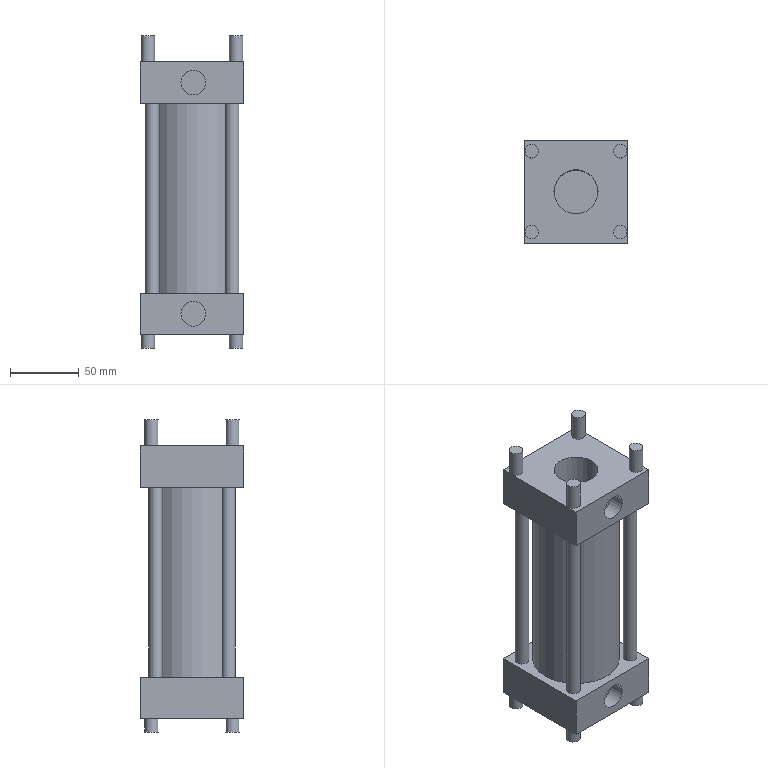Part | NX | features solid 2 | 1 solid | 39 faces | box 75 x 75 x 227 mm | volume 665796 mm3 | plane 23 | cylinder 16 | commonest cylinder face diameters 9.874 x12 18 x2 32 x1 63 x1
STEP:
#1=CARTESIAN_POINT('',(-34.06,-86.406,-135.));
#2=VERTEX_POINT('',#1);
#3=CARTESIAN_POINT('',(-29.124,-86.406,-135.));
#4=DIRECTION('',(0.,0.,-1.));
#5=DIRECTION('',(-1.,0.,0.));
#6=AXIS2_PLACEMENT_3D('',#3,#4,#5);
#7=CIRCLE('',#6,4.937);
#8=EDGE_CURVE('',#2,#2,#7,.T.);
#9=ORIENTED_EDGE('',*,*,#8,.F.);
#10=EDGE_LOOP('',(#9));
#11=FACE_BOUND('',#10,.T.);
#12=CARTESIAN_POINT('',(-24.187,-33.594,-135.));
#13=VERTEX_POINT('',#12);
#14=CARTESIAN_POINT('',(-29.124,-33.594,-135.));
#15=DIRECTION('',(0.,0.,1.));
#16=DIRECTION('',(1.,0.,0.));
#17=AXIS2_PLACEMENT_3D('',#14,#15,#16);
#18=CIRCLE('',#17,4.937);
#19=EDGE_CURVE('',#13,#13,#18,.T.);
#20=ORIENTED_EDGE('',*,*,#19,.T.);
#21=EDGE_LOOP('',(#20));
#22=FACE_BOUND('',#21,.T.);
#23=CARTESIAN_POINT('',(37.5,-97.5,-135.));
#24=VERTEX_POINT('',#23);
#25=CARTESIAN_POINT('',(-37.5,-97.5,-135.));
#26=VERTEX_POINT('',#25);
#27=CARTESIAN_POINT('',(-41.,-97.5,-135.));
#28=DIRECTION('',(-1.,0.,0.));
#29=VECTOR('',#28,1000.);
#30=LINE('',#27,#29);
#31=EDGE_CURVE('',#24,#26,#30,.T.);
#32=ORIENTED_EDGE('',*,*,#31,.T.);
#33=CARTESIAN_POINT('',(-37.5,-22.5,-135.));
#34=VERTEX_POINT('',#33);
#35=CARTESIAN_POINT('',(-37.5,-60.,-135.));
#36=DIRECTION('',(0.,1.,0.));
#37=VECTOR('',#36,1000.);
#38=LINE('',#35,#37);
#39=EDGE_CURVE('',#26,#34,#38,.T.);
#40=ORIENTED_EDGE('',*,*,#39,.T.);
#41=CARTESIAN_POINT('',(37.5,-22.5,-135.));
#42=VERTEX_POINT('',#41);
#43=CARTESIAN_POINT('',(-41.,-22.5,-135.));
#44=DIRECTION('',(-1.,0.,0.));
#45=VECTOR('',#44,1000.);
#46=LINE('',#43,#45);
#47=EDGE_CURVE('',#42,#34,#46,.T.);
#48=ORIENTED_EDGE('',*,*,#47,.F.);
#49=CARTESIAN_POINT('',(37.5,-60.,-135.));
#50=DIRECTION('',(0.,-1.,0.));
#51=VECTOR('',#50,1000.);
#52=LINE('',#49,#51);
#53=EDGE_CURVE('',#42,#24,#52,.T.);
#54=ORIENTED_EDGE('',*,*,#53,.T.);
#55=EDGE_LOOP('',(#32,#40,#48,#54));
#56=FACE_BOUND('',#55,.T.);
#57=CARTESIAN_POINT('',(34.06,-33.594,-135.));
#58=VERTEX_POINT('',#57);
#59=CARTESIAN_POINT('',(29.124,-33.594,-135.));
#60=DIRECTION('',(0.,0.,-1.));
#61=DIRECTION('',(1.,0.,0.));
#62=AXIS2_PLACEMENT_3D('',#59,#60,#61);
#63=CIRCLE('',#62,4.937);
#64=EDGE_CURVE('',#58,#58,#63,.T.);
#65=ORIENTED_EDGE('',*,*,#64,.F.);
#66=EDGE_LOOP('',(#65));
#67=FACE_BOUND('',#66,.T.);
#68=CARTESIAN_POINT('',(34.06,-86.406,-135.));
#69=VERTEX_POINT('',#68);
#70=CARTESIAN_POINT('',(29.124,-86.406,-135.));
#71=DIRECTION('',(0.,0.,1.));
#72=DIRECTION('',(1.,0.,0.));
#73=AXIS2_PLACEMENT_3D('',#70,#71,#72);
#74=CIRCLE('',#73,4.937);
#75=EDGE_CURVE('',#69,#69,#74,.T.);
#76=ORIENTED_EDGE('',*,*,#75,.T.);
#77=EDGE_LOOP('',(#76));
#78=FACE_BOUND('',#77,.T.);
#79=CARTESIAN_POINT('',(31.5,-60.,-135.));
#80=VERTEX_POINT('',#79);
#81=CARTESIAN_POINT('',(0.,-60.,-135.));
#82=DIRECTION('',(0.,0.,1.));
#83=DIRECTION('',(1.,0.,0.));
#84=AXIS2_PLACEMENT_3D('',#81,#82,#83);
#85=CIRCLE('',#84,31.5);
#86=EDGE_CURVE('',#80,#80,#85,.F.);
#87=ORIENTED_EDGE('',*,*,#86,.F.);
#88=EDGE_LOOP('',(#87));
#89=FACE_BOUND('',#88,.T.);
#90=CARTESIAN_POINT('',(-41.,-101.,-135.));
#91=DIRECTION('',(0.,0.,1.));
#92=DIRECTION('',(1.,0.,0.));
#93=AXIS2_PLACEMENT_3D('',#90,#91,#92);
#94=PLANE('',#93);
#95=ADVANCED_FACE('',(#11,#22,#56,#67,#78,#89),#94,.F.);
#96=CARTESIAN_POINT('',(-8.,-97.5,-120.));
#97=VERTEX_POINT('',#96);
#98=CARTESIAN_POINT('',(1.,-97.5,-120.));
#99=DIRECTION('',(0.,1.,0.));
#100=DIRECTION('',(-1.,0.,0.));
#101=AXIS2_PLACEMENT_3D('',#98,#99,#100);
#102=CIRCLE('',#101,9.);
#103=EDGE_CURVE('',#97,#97,#102,.T.);
#104=ORIENTED_EDGE('',*,*,#103,.T.);
#105=EDGE_LOOP('',(#104));
#106=FACE_BOUND('',#105,.T.);
#107=CARTESIAN_POINT('',(37.5,-97.5,-105.));
#108=VERTEX_POINT('',#107);
#109=CARTESIAN_POINT('',(-37.5,-97.5,-105.));
#110=VERTEX_POINT('',#109);
#111=CARTESIAN_POINT('',(-41.,-97.5,-105.));
#112=DIRECTION('',(-1.,0.,0.));
#113=VECTOR('',#112,1000.);
#114=LINE('',#111,#113);
#115=EDGE_CURVE('',#108,#110,#114,.T.);
#116=ORIENTED_EDGE('',*,*,#115,.T.);
#117=CARTESIAN_POINT('',(-37.5,-97.5,-135.));
#118=DIRECTION('',(0.,0.,1.));
#119=VECTOR('',#118,1000.);
#120=LINE('',#117,#119);
#121=EDGE_CURVE('',#26,#110,#120,.T.);
#122=ORIENTED_EDGE('',*,*,#121,.F.);
#123=ORIENTED_EDGE('',*,*,#31,.F.);
#124=CARTESIAN_POINT('',(37.5,-97.5,-135.));
#125=DIRECTION('',(0.,0.,1.));
#126=VECTOR('',#125,1000.);
#127=LINE('',#124,#126);
#128=EDGE_CURVE('',#24,#108,#127,.T.);
#129=ORIENTED_EDGE('',*,*,#128,.T.);
#130=EDGE_LOOP('',(#116,#122,#123,#129));
#131=FACE_BOUND('',#130,.T.);
#132=CARTESIAN_POINT('',(41.,-97.5,-135.));
#133=DIRECTION('',(0.,1.,0.));
#134=DIRECTION('',(-1.,0.,0.));
#135=AXIS2_PLACEMENT_3D('',#132,#133,#134);
#136=PLANE('',#135);
#137=ADVANCED_FACE('',(#106,#131),#136,.F.);
#138=CARTESIAN_POINT('',(37.5,-22.5,-105.));
#139=VERTEX_POINT('',#138);
#140=CARTESIAN_POINT('',(37.5,-101.,-105.));
#141=DIRECTION('',(0.,1.,0.));
#142=VECTOR('',#141,1000.);
#143=LINE('',#140,#142);
#144=EDGE_CURVE('',#108,#139,#143,.T.);
#145=ORIENTED_EDGE('',*,*,#144,.F.);
#146=ORIENTED_EDGE('',*,*,#128,.F.);
#147=ORIENTED_EDGE('',*,*,#53,.F.);
#148=CARTESIAN_POINT('',(37.5,-22.5,-135.));
#149=DIRECTION('',(0.,0.,1.));
#150=VECTOR('',#149,1000.);
#151=LINE('',#148,#150);
#152=EDGE_CURVE('',#42,#139,#151,.T.);
#153=ORIENTED_EDGE('',*,*,#152,.T.);
#154=EDGE_LOOP('',(#145,#146,#147,#153));
#155=FACE_BOUND('',#154,.T.);
#156=CARTESIAN_POINT('',(37.5,-60.,-135.));
#157=DIRECTION('',(1.,0.,0.));
#158=DIRECTION('',(0.,1.,0.));
#159=AXIS2_PLACEMENT_3D('',#156,#157,#158);
#160=PLANE('',#159);
#161=ADVANCED_FACE('',(#155),#160,.T.);
#162=CARTESIAN_POINT('',(-37.5,-22.5,-105.));
#163=VERTEX_POINT('',#162);
#164=CARTESIAN_POINT('',(-41.,-22.5,-105.));
#165=DIRECTION('',(1.,0.,0.));
#166=VECTOR('',#165,1000.);
#167=LINE('',#164,#166);
#168=EDGE_CURVE('',#163,#139,#167,.T.);
#169=ORIENTED_EDGE('',*,*,#168,.T.);
#170=ORIENTED_EDGE('',*,*,#152,.F.);
#171=ORIENTED_EDGE('',*,*,#47,.T.);
#172=CARTESIAN_POINT('',(-37.5,-22.5,-135.));
#173=DIRECTION('',(0.,0.,1.));
#174=VECTOR('',#173,1000.);
#175=LINE('',#172,#174);
#176=EDGE_CURVE('',#34,#163,#175,.T.);
#177=ORIENTED_EDGE('',*,*,#176,.T.);
#178=EDGE_LOOP('',(#169,#170,#171,#177));
#179=FACE_BOUND('',#178,.T.);
#180=CARTESIAN_POINT('',(-41.,-22.5,-135.));
#181=DIRECTION('',(0.,-1.,0.));
#182=DIRECTION('',(0.,0.,-1.));
#183=AXIS2_PLACEMENT_3D('',#180,#181,#182);
#184=PLANE('',#183);
#185=ADVANCED_FACE('',(#179),#184,.F.);
#186=CARTESIAN_POINT('',(-37.5,-101.,-105.));
#187=DIRECTION('',(0.,-1.,0.));
#188=VECTOR('',#187,1000.);
#189=LINE('',#186,#188);
#190=EDGE_CURVE('',#163,#110,#189,.T.);
#191=ORIENTED_EDGE('',*,*,#190,.F.);
#192=ORIENTED_EDGE('',*,*,#176,.F.);
#193=ORIENTED_EDGE('',*,*,#39,.F.);
#194=ORIENTED_EDGE('',*,*,#121,.T.);
#195=EDGE_LOOP('',(#191,#192,#193,#194));
#196=FACE_BOUND('',#195,.T.);
#197=CARTESIAN_POINT('',(-37.5,-60.,-135.));
#198=DIRECTION('',(-1.,0.,0.));
#199=DIRECTION('',(0.,-1.,0.));
#200=AXIS2_PLACEMENT_3D('',#197,#198,#199);
#201=PLANE('',#200);
#202=ADVANCED_FACE('',(#196),#201,.T.);
#203=CARTESIAN_POINT('',(16.,-60.,-105.));
#204=VERTEX_POINT('',#203);
#205=CARTESIAN_POINT('',(0.,-60.,-105.));
#206=DIRECTION('',(0.,0.,1.));
#207=DIRECTION('',(1.,0.,0.));
#208=AXIS2_PLACEMENT_3D('',#205,#206,#207);
#209=CIRCLE('',#208,16.);
#210=EDGE_CURVE('',#204,#204,#209,.T.);
#211=ORIENTED_EDGE('',*,*,#210,.F.);
#212=EDGE_LOOP('',(#211));
#213=FACE_BOUND('',#212,.T.);
#214=CARTESIAN_POINT('',(37.06,-89.406,-105.));
#215=VERTEX_POINT('',#214);
#216=CARTESIAN_POINT('',(32.124,-89.406,-105.));
#217=DIRECTION('',(0.,0.,1.));
#218=DIRECTION('',(1.,0.,0.));
#219=AXIS2_PLACEMENT_3D('',#216,#217,#218);
#220=CIRCLE('',#219,4.937);
#221=EDGE_CURVE('',#215,#215,#220,.T.);
#222=ORIENTED_EDGE('',*,*,#221,.F.);
#223=EDGE_LOOP('',(#222));
#224=FACE_BOUND('',#223,.T.);
#225=CARTESIAN_POINT('',(37.06,-30.594,-105.));
#226=VERTEX_POINT('',#225);
#227=CARTESIAN_POINT('',(32.124,-30.594,-105.));
#228=DIRECTION('',(0.,0.,1.));
#229=DIRECTION('',(1.,0.,0.));
#230=AXIS2_PLACEMENT_3D('',#227,#228,#229);
#231=CIRCLE('',#230,4.937);
#232=EDGE_CURVE('',#226,#226,#231,.F.);
#233=ORIENTED_EDGE('',*,*,#232,.T.);
#234=EDGE_LOOP('',(#233));
#235=FACE_BOUND('',#234,.T.);
#236=ORIENTED_EDGE('',*,*,#190,.T.);
#237=ORIENTED_EDGE('',*,*,#115,.F.);
#238=ORIENTED_EDGE('',*,*,#144,.T.);
#239=ORIENTED_EDGE('',*,*,#168,.F.);
#240=EDGE_LOOP('',(#236,#237,#238,#239));
#241=FACE_BOUND('',#240,.T.);
#242=CARTESIAN_POINT('',(-37.06,-30.594,-105.));
#243=VERTEX_POINT('',#242);
#244=CARTESIAN_POINT('',(-32.124,-30.594,-105.));
#245=DIRECTION('',(0.,0.,1.));
#246=DIRECTION('',(-1.,0.,0.));
#247=AXIS2_PLACEMENT_3D('',#244,#245,#246);
#248=CIRCLE('',#247,4.937);
#249=EDGE_CURVE('',#243,#243,#248,.T.);
#250=ORIENTED_EDGE('',*,*,#249,.F.);
#251=EDGE_LOOP('',(#250));
#252=FACE_BOUND('',#251,.T.);
#253=CARTESIAN_POINT('',(-27.187,-89.406,-105.));
#254=VERTEX_POINT('',#253);
#255=CARTESIAN_POINT('',(-32.124,-89.406,-105.));
#256=DIRECTION('',(0.,0.,1.));
#257=DIRECTION('',(1.,0.,0.));
#258=AXIS2_PLACEMENT_3D('',#255,#256,#257);
#259=CIRCLE('',#258,4.937);
#260=EDGE_CURVE('',#254,#254,#259,.F.);
#261=ORIENTED_EDGE('',*,*,#260,.T.);
#262=EDGE_LOOP('',(#261));
#263=FACE_BOUND('',#262,.T.);
#264=CARTESIAN_POINT('',(-41.,-101.,-105.));
#265=DIRECTION('',(0.,0.,1.));
#266=DIRECTION('',(1.,0.,0.));
#267=AXIS2_PLACEMENT_3D('',#264,#265,#266);
#268=PLANE('',#267);
#269=ADVANCED_FACE('',(#213,#224,#235,#241,#252,#263),#268,.T.);
#270=CARTESIAN_POINT('',(37.06,-30.594,-86.));
#271=VERTEX_POINT('',#270);
#272=CARTESIAN_POINT('',(32.124,-30.594,-86.));
#273=DIRECTION('',(0.,0.,-1.));
#274=DIRECTION('',(1.,0.,0.));
#275=AXIS2_PLACEMENT_3D('',#272,#273,#274);
#276=CIRCLE('',#275,4.937);
#277=EDGE_CURVE('',#271,#271,#276,.T.);
#278=ORIENTED_EDGE('',*,*,#277,.F.);
#279=EDGE_LOOP('',(#278));
#280=FACE_BOUND('',#279,.T.);
#281=CARTESIAN_POINT('',(32.124,-30.594,-86.));
#282=DIRECTION('',(0.,0.,-1.));
#283=DIRECTION('',(-1.,0.,0.));
#284=AXIS2_PLACEMENT_3D('',#281,#282,#283);
#285=PLANE('',#284);
#286=ADVANCED_FACE('',(#280),#285,.F.);
#287=ORIENTED_EDGE('',*,*,#232,.F.);
#288=EDGE_LOOP('',(#287));
#289=FACE_BOUND('',#288,.T.);
#290=ORIENTED_EDGE('',*,*,#277,.T.);
#291=EDGE_LOOP('',(#290));
#292=FACE_BOUND('',#291,.T.);
#293=CARTESIAN_POINT('',(32.124,-30.594,-313.));
#294=DIRECTION('',(0.,0.,1.));
#295=DIRECTION('',(1.,0.,0.));
#296=AXIS2_PLACEMENT_3D('',#293,#294,#295);
#297=CYLINDRICAL_SURFACE('',#296,4.937);
#298=ADVANCED_FACE('',(#289,#292),#297,.T.);
#299=CARTESIAN_POINT('',(34.06,-33.594,-273.));
#300=VERTEX_POINT('',#299);
#301=CARTESIAN_POINT('',(29.124,-33.594,-273.));
#302=DIRECTION('',(0.,0.,-1.));
#303=DIRECTION('',(1.,0.,0.));
#304=AXIS2_PLACEMENT_3D('',#301,#302,#303);
#305=CIRCLE('',#304,4.937);
#306=EDGE_CURVE('',#300,#300,#305,.T.);
#307=ORIENTED_EDGE('',*,*,#306,.F.);
#308=EDGE_LOOP('',(#307));
#309=FACE_BOUND('',#308,.T.);
#310=ORIENTED_EDGE('',*,*,#64,.T.);
#311=EDGE_LOOP('',(#310));
#312=FACE_BOUND('',#311,.T.);
#313=CARTESIAN_POINT('',(29.124,-33.594,-313.));
#314=DIRECTION('',(0.,0.,1.));
#315=DIRECTION('',(1.,0.,0.));
#316=AXIS2_PLACEMENT_3D('',#313,#314,#315);
#317=CYLINDRICAL_SURFACE('',#316,4.937);
#318=ADVANCED_FACE('',(#309,#312),#317,.T.);
#319=CARTESIAN_POINT('',(-37.06,-30.594,-86.));
#320=VERTEX_POINT('',#319);
#321=CARTESIAN_POINT('',(-32.124,-30.594,-86.));
#322=DIRECTION('',(0.,0.,1.));
#323=DIRECTION('',(-1.,0.,0.));
#324=AXIS2_PLACEMENT_3D('',#321,#322,#323);
#325=CIRCLE('',#324,4.937);
#326=EDGE_CURVE('',#320,#320,#325,.T.);
#327=ORIENTED_EDGE('',*,*,#326,.T.);
#328=EDGE_LOOP('',(#327));
#329=FACE_BOUND('',#328,.T.);
#330=CARTESIAN_POINT('',(-32.124,-30.594,-86.));
#331=DIRECTION('',(0.,0.,1.));
#332=DIRECTION('',(1.,0.,0.));
#333=AXIS2_PLACEMENT_3D('',#330,#331,#332);
#334=PLANE('',#333);
#335=ADVANCED_FACE('',(#329),#334,.T.);
#336=ORIENTED_EDGE('',*,*,#249,.T.);
#337=EDGE_LOOP('',(#336));
#338=FACE_BOUND('',#337,.T.);
#339=ORIENTED_EDGE('',*,*,#326,.F.);
#340=EDGE_LOOP('',(#339));
#341=FACE_BOUND('',#340,.T.);
#342=CARTESIAN_POINT('',(-32.124,-30.594,-313.));
#343=DIRECTION('',(0.,0.,1.));
#344=DIRECTION('',(1.,0.,0.));
#345=AXIS2_PLACEMENT_3D('',#342,#343,#344);
#346=CYLINDRICAL_SURFACE('',#345,4.937);
#347=ADVANCED_FACE('',(#338,#341),#346,.T.);
#348=CARTESIAN_POINT('',(-24.187,-33.594,-273.));
#349=VERTEX_POINT('',#348);
#350=CARTESIAN_POINT('',(-29.124,-33.594,-273.));
#351=DIRECTION('',(0.,0.,1.));
#352=DIRECTION('',(1.,0.,0.));
#353=AXIS2_PLACEMENT_3D('',#350,#351,#352);
#354=CIRCLE('',#353,4.937);
#355=EDGE_CURVE('',#349,#349,#354,.F.);
#356=ORIENTED_EDGE('',*,*,#355,.F.);
#357=EDGE_LOOP('',(#356));
#358=FACE_BOUND('',#357,.T.);
#359=ORIENTED_EDGE('',*,*,#19,.F.);
#360=EDGE_LOOP('',(#359));
#361=FACE_BOUND('',#360,.T.);
#362=CARTESIAN_POINT('',(-29.124,-33.594,-313.));
#363=DIRECTION('',(0.,0.,1.));
#364=DIRECTION('',(1.,0.,0.));
#365=AXIS2_PLACEMENT_3D('',#362,#363,#364);
#366=CYLINDRICAL_SURFACE('',#365,4.937);
#367=ADVANCED_FACE('',(#358,#361),#366,.T.);
#368=CARTESIAN_POINT('',(-37.06,-89.406,-86.));
#369=VERTEX_POINT('',#368);
#370=CARTESIAN_POINT('',(-32.124,-89.406,-86.));
#371=DIRECTION('',(0.,0.,-1.));
#372=DIRECTION('',(-1.,0.,0.));
#373=AXIS2_PLACEMENT_3D('',#370,#371,#372);
#374=CIRCLE('',#373,4.937);
#375=EDGE_CURVE('',#369,#369,#374,.T.);
#376=ORIENTED_EDGE('',*,*,#375,.F.);
#377=EDGE_LOOP('',(#376));
#378=FACE_BOUND('',#377,.T.);
#379=CARTESIAN_POINT('',(-32.124,-89.406,-86.));
#380=DIRECTION('',(0.,0.,-1.));
#381=DIRECTION('',(-1.,0.,0.));
#382=AXIS2_PLACEMENT_3D('',#379,#380,#381);
#383=PLANE('',#382);
#384=ADVANCED_FACE('',(#378),#383,.F.);
#385=ORIENTED_EDGE('',*,*,#260,.F.);
#386=EDGE_LOOP('',(#385));
#387=FACE_BOUND('',#386,.T.);
#388=ORIENTED_EDGE('',*,*,#375,.T.);
#389=EDGE_LOOP('',(#388));
#390=FACE_BOUND('',#389,.T.);
#391=CARTESIAN_POINT('',(-32.124,-89.406,-313.));
#392=DIRECTION('',(0.,0.,1.));
#393=DIRECTION('',(1.,0.,0.));
#394=AXIS2_PLACEMENT_3D('',#391,#392,#393);
#395=CYLINDRICAL_SURFACE('',#394,4.937);
#396=ADVANCED_FACE('',(#387,#390),#395,.T.);
#397=CARTESIAN_POINT('',(-34.06,-86.406,-273.));
#398=VERTEX_POINT('',#397);
#399=CARTESIAN_POINT('',(-29.124,-86.406,-273.));
#400=DIRECTION('',(0.,0.,-1.));
#401=DIRECTION('',(-1.,0.,0.));
#402=AXIS2_PLACEMENT_3D('',#399,#400,#401);
#403=CIRCLE('',#402,4.937);
#404=EDGE_CURVE('',#398,#398,#403,.T.);
#405=ORIENTED_EDGE('',*,*,#404,.F.);
#406=EDGE_LOOP('',(#405));
#407=FACE_BOUND('',#406,.T.);
#408=ORIENTED_EDGE('',*,*,#8,.T.);
#409=EDGE_LOOP('',(#408));
#410=FACE_BOUND('',#409,.T.);
#411=CARTESIAN_POINT('',(-29.124,-86.406,-313.));
#412=DIRECTION('',(0.,0.,1.));
#413=DIRECTION('',(1.,0.,0.));
#414=AXIS2_PLACEMENT_3D('',#411,#412,#413);
#415=CYLINDRICAL_SURFACE('',#414,4.937);
#416=ADVANCED_FACE('',(#407,#410),#415,.T.);
#417=CARTESIAN_POINT('',(37.06,-89.406,-86.));
#418=VERTEX_POINT('',#417);
#419=CARTESIAN_POINT('',(32.124,-89.406,-86.));
#420=DIRECTION('',(0.,0.,1.));
#421=DIRECTION('',(1.,0.,0.));
#422=AXIS2_PLACEMENT_3D('',#419,#420,#421);
#423=CIRCLE('',#422,4.937);
#424=EDGE_CURVE('',#418,#418,#423,.T.);
#425=ORIENTED_EDGE('',*,*,#424,.T.);
#426=EDGE_LOOP('',(#425));
#427=FACE_BOUND('',#426,.T.);
#428=CARTESIAN_POINT('',(32.124,-89.406,-86.));
#429=DIRECTION('',(0.,0.,1.));
#430=DIRECTION('',(1.,0.,0.));
#431=AXIS2_PLACEMENT_3D('',#428,#429,#430);
#432=PLANE('',#431);
#433=ADVANCED_FACE('',(#427),#432,.T.);
#434=ORIENTED_EDGE('',*,*,#221,.T.);
#435=EDGE_LOOP('',(#434));
#436=FACE_BOUND('',#435,.T.);
#437=ORIENTED_EDGE('',*,*,#424,.F.);
#438=EDGE_LOOP('',(#437));
#439=FACE_BOUND('',#438,.T.);
#440=CARTESIAN_POINT('',(32.124,-89.406,-313.));
#441=DIRECTION('',(0.,0.,1.));
#442=DIRECTION('',(1.,0.,0.));
#443=AXIS2_PLACEMENT_3D('',#440,#441,#442);
#444=CYLINDRICAL_SURFACE('',#443,4.937);
#445=ADVANCED_FACE('',(#436,#439),#444,.T.);
#446=CARTESIAN_POINT('',(34.06,-86.406,-273.));
#447=VERTEX_POINT('',#446);
#448=CARTESIAN_POINT('',(29.124,-86.406,-273.));
#449=DIRECTION('',(0.,0.,1.));
#450=DIRECTION('',(1.,0.,0.));
#451=AXIS2_PLACEMENT_3D('',#448,#449,#450);
#452=CIRCLE('',#451,4.937);
#453=EDGE_CURVE('',#447,#447,#452,.F.);
#454=ORIENTED_EDGE('',*,*,#453,.F.);
#455=EDGE_LOOP('',(#454));
#456=FACE_BOUND('',#455,.T.);
#457=ORIENTED_EDGE('',*,*,#75,.F.);
#458=EDGE_LOOP('',(#457));
#459=FACE_BOUND('',#458,.T.);
#460=CARTESIAN_POINT('',(29.124,-86.406,-313.));
#461=DIRECTION('',(0.,0.,1.));
#462=DIRECTION('',(1.,0.,0.));
#463=AXIS2_PLACEMENT_3D('',#460,#461,#462);
#464=CYLINDRICAL_SURFACE('',#463,4.937);
#465=ADVANCED_FACE('',(#456,#459),#464,.T.);
#466=ORIENTED_EDGE('',*,*,#210,.T.);
#467=EDGE_LOOP('',(#466));
#468=FACE_BOUND('',#467,.T.);
#469=CARTESIAN_POINT('',(16.,-60.,-288.));
#470=VERTEX_POINT('',#469);
#471=CARTESIAN_POINT('',(0.,-60.,-288.));
#472=DIRECTION('',(0.,0.,1.));
#473=DIRECTION('',(1.,0.,0.));
#474=AXIS2_PLACEMENT_3D('',#471,#472,#473);
#475=CIRCLE('',#474,16.);
#476=EDGE_CURVE('',#470,#470,#475,.T.);
#477=ORIENTED_EDGE('',*,*,#476,.F.);
#478=EDGE_LOOP('',(#477));
#479=FACE_BOUND('',#478,.T.);
#480=CARTESIAN_POINT('',(0.,-60.,-238.));
#481=DIRECTION('',(0.,0.,1.));
#482=DIRECTION('',(1.,0.,0.));
#483=AXIS2_PLACEMENT_3D('',#480,#481,#482);
#484=CYLINDRICAL_SURFACE('',#483,16.);
#485=ADVANCED_FACE('',(#468,#479),#484,.F.);
#486=CARTESIAN_POINT('',(-8.,-86.,-120.));
#487=VERTEX_POINT('',#486);
#488=CARTESIAN_POINT('',(1.,-86.,-120.));
#489=DIRECTION('',(0.,1.,0.));
#490=DIRECTION('',(-1.,0.,0.));
#491=AXIS2_PLACEMENT_3D('',#488,#489,#490);
#492=CIRCLE('',#491,9.);
#493=EDGE_CURVE('',#487,#487,#492,.T.);
#494=ORIENTED_EDGE('',*,*,#493,.F.);
#495=EDGE_LOOP('',(#494));
#496=FACE_BOUND('',#495,.T.);
#497=CARTESIAN_POINT('',(1.,-86.,-120.));
#498=DIRECTION('',(0.,1.,0.));
#499=DIRECTION('',(-1.,0.,0.));
#500=AXIS2_PLACEMENT_3D('',#497,#498,#499);
#501=PLANE('',#500);
#502=ADVANCED_FACE('',(#496),#501,.F.);
#503=ORIENTED_EDGE('',*,*,#493,.T.);
#504=EDGE_LOOP('',(#503));
#505=FACE_BOUND('',#504,.T.);
#506=ORIENTED_EDGE('',*,*,#103,.F.);
#507=EDGE_LOOP('',(#506));
#508=FACE_BOUND('',#507,.T.);
#509=CARTESIAN_POINT('',(1.,-101.,-120.));
#510=DIRECTION('',(0.,1.,0.));
#511=DIRECTION('',(-1.,0.,0.));
#512=AXIS2_PLACEMENT_3D('',#509,#510,#511);
#513=CYLINDRICAL_SURFACE('',#512,9.);
#514=ADVANCED_FACE('',(#505,#508),#513,.F.);
#515=ORIENTED_EDGE('',*,*,#476,.T.);
#516=EDGE_LOOP('',(#515));
#517=FACE_BOUND('',#516,.T.);
#518=CARTESIAN_POINT('',(0.,-60.,-288.));
#519=DIRECTION('',(0.,0.,1.));
#520=DIRECTION('',(1.,0.,0.));
#521=AXIS2_PLACEMENT_3D('',#518,#519,#520);
#522=PLANE('',#521);
#523=ADVANCED_FACE('',(#517),#522,.T.);
#524=ORIENTED_EDGE('',*,*,#306,.T.);
#525=EDGE_LOOP('',(#524));
#526=FACE_BOUND('',#525,.T.);
#527=ORIENTED_EDGE('',*,*,#355,.T.);
#528=EDGE_LOOP('',(#527));
#529=FACE_BOUND('',#528,.T.);
#530=CARTESIAN_POINT('',(-37.5,-97.5,-273.));
#531=VERTEX_POINT('',#530);
#532=CARTESIAN_POINT('',(-37.5,-22.5,-273.));
#533=VERTEX_POINT('',#532);
#534=CARTESIAN_POINT('',(-37.5,-101.,-273.));
#535=DIRECTION('',(0.,1.,0.));
#536=VECTOR('',#535,1000.);
#537=LINE('',#534,#536);
#538=EDGE_CURVE('',#531,#533,#537,.T.);
#539=ORIENTED_EDGE('',*,*,#538,.F.);
#540=CARTESIAN_POINT('',(37.5,-97.5,-273.));
#541=VERTEX_POINT('',#540);
#542=CARTESIAN_POINT('',(41.,-97.5,-273.));
#543=DIRECTION('',(-1.,0.,0.));
#544=VECTOR('',#543,1000.);
#545=LINE('',#542,#544);
#546=EDGE_CURVE('',#541,#531,#545,.T.);
#547=ORIENTED_EDGE('',*,*,#546,.F.);
#548=CARTESIAN_POINT('',(37.5,-22.5,-273.));
#549=VERTEX_POINT('',#548);
#550=CARTESIAN_POINT('',(37.5,-101.,-273.));
#551=DIRECTION('',(0.,-1.,0.));
#552=VECTOR('',#551,1000.);
#553=LINE('',#550,#552);
#554=EDGE_CURVE('',#549,#541,#553,.T.);
#555=ORIENTED_EDGE('',*,*,#554,.F.);
#556=CARTESIAN_POINT('',(-41.,-22.5,-273.));
#557=DIRECTION('',(-1.,0.,0.));
#558=VECTOR('',#557,1000.);
#559=LINE('',#556,#558);
#560=EDGE_CURVE('',#549,#533,#559,.T.);
#561=ORIENTED_EDGE('',*,*,#560,.T.);
#562=EDGE_LOOP('',(#539,#547,#555,#561));
#563=FACE_BOUND('',#562,.T.);
#564=ORIENTED_EDGE('',*,*,#453,.T.);
#565=EDGE_LOOP('',(#564));
#566=FACE_BOUND('',#565,.T.);
#567=ORIENTED_EDGE('',*,*,#404,.T.);
#568=EDGE_LOOP('',(#567));
#569=FACE_BOUND('',#568,.T.);
#570=CARTESIAN_POINT('',(31.5,-60.,-273.));
#571=VERTEX_POINT('',#570);
#572=CARTESIAN_POINT('',(0.,-60.,-273.));
#573=DIRECTION('',(0.,0.,1.));
#574=DIRECTION('',(1.,0.,0.));
#575=AXIS2_PLACEMENT_3D('',#572,#573,#574);
#576=CIRCLE('',#575,31.5);
#577=EDGE_CURVE('',#571,#571,#576,.F.);
#578=ORIENTED_EDGE('',*,*,#577,.T.);
#579=EDGE_LOOP('',(#578));
#580=FACE_BOUND('',#579,.T.);
#581=CARTESIAN_POINT('',(-41.,-101.,-273.));
#582=DIRECTION('',(0.,0.,1.));
#583=DIRECTION('',(1.,0.,0.));
#584=AXIS2_PLACEMENT_3D('',#581,#582,#583);
#585=PLANE('',#584);
#586=ADVANCED_FACE('',(#526,#529,#563,#566,#569,#580),#585,.T.);
#587=CARTESIAN_POINT('',(10.,-97.5,-288.));
#588=VERTEX_POINT('',#587);
#589=CARTESIAN_POINT('',(1.,-97.5,-288.));
#590=DIRECTION('',(0.,-1.,0.));
#591=DIRECTION('',(1.,0.,0.));
#592=AXIS2_PLACEMENT_3D('',#589,#590,#591);
#593=CIRCLE('',#592,9.);
#594=EDGE_CURVE('',#588,#588,#593,.F.);
#595=ORIENTED_EDGE('',*,*,#594,.T.);
#596=EDGE_LOOP('',(#595));
#597=FACE_BOUND('',#596,.T.);
#598=CARTESIAN_POINT('',(37.5,-97.5,-303.));
#599=VERTEX_POINT('',#598);
#600=CARTESIAN_POINT('',(-37.5,-97.5,-303.));
#601=VERTEX_POINT('',#600);
#602=CARTESIAN_POINT('',(41.,-97.5,-303.));
#603=DIRECTION('',(-1.,0.,0.));
#604=VECTOR('',#603,1000.);
#605=LINE('',#602,#604);
#606=EDGE_CURVE('',#599,#601,#605,.T.);
#607=ORIENTED_EDGE('',*,*,#606,.F.);
#608=CARTESIAN_POINT('',(37.5,-97.5,-273.));
#609=DIRECTION('',(0.,0.,-1.));
#610=VECTOR('',#609,1000.);
#611=LINE('',#608,#610);
#612=EDGE_CURVE('',#541,#599,#611,.T.);
#613=ORIENTED_EDGE('',*,*,#612,.F.);
#614=ORIENTED_EDGE('',*,*,#546,.T.);
#615=CARTESIAN_POINT('',(-37.5,-97.5,-273.));
#616=DIRECTION('',(0.,0.,-1.));
#617=VECTOR('',#616,1000.);
#618=LINE('',#615,#617);
#619=EDGE_CURVE('',#531,#601,#618,.T.);
#620=ORIENTED_EDGE('',*,*,#619,.T.);
#621=EDGE_LOOP('',(#607,#613,#614,#620));
#622=FACE_BOUND('',#621,.T.);
#623=CARTESIAN_POINT('',(41.,-97.5,-273.));
#624=DIRECTION('',(0.,-1.,0.));
#625=DIRECTION('',(1.,0.,0.));
#626=AXIS2_PLACEMENT_3D('',#623,#624,#625);
#627=PLANE('',#626);
#628=ADVANCED_FACE('',(#597,#622),#627,.T.);
#629=CARTESIAN_POINT('',(37.5,-22.5,-303.));
#630=VERTEX_POINT('',#629);
#631=CARTESIAN_POINT('',(37.5,-60.,-303.));
#632=DIRECTION('',(0.,1.,0.));
#633=VECTOR('',#632,1000.);
#634=LINE('',#631,#633);
#635=EDGE_CURVE('',#599,#630,#634,.T.);
#636=ORIENTED_EDGE('',*,*,#635,.T.);
#637=CARTESIAN_POINT('',(37.5,-22.5,-273.));
#638=DIRECTION('',(0.,0.,-1.));
#639=VECTOR('',#638,1000.);
#640=LINE('',#637,#639);
#641=EDGE_CURVE('',#549,#630,#640,.T.);
#642=ORIENTED_EDGE('',*,*,#641,.F.);
#643=ORIENTED_EDGE('',*,*,#554,.T.);
#644=ORIENTED_EDGE('',*,*,#612,.T.);
#645=EDGE_LOOP('',(#636,#642,#643,#644));
#646=FACE_BOUND('',#645,.T.);
#647=CARTESIAN_POINT('',(37.5,-60.,-273.));
#648=DIRECTION('',(-1.,0.,0.));
#649=DIRECTION('',(0.,-1.,0.));
#650=AXIS2_PLACEMENT_3D('',#647,#648,#649);
#651=PLANE('',#650);
#652=ADVANCED_FACE('',(#646),#651,.F.);
#653=CARTESIAN_POINT('',(-37.5,-22.5,-303.));
#654=VERTEX_POINT('',#653);
#655=CARTESIAN_POINT('',(-41.,-22.5,-303.));
#656=DIRECTION('',(1.,0.,0.));
#657=VECTOR('',#656,1000.);
#658=LINE('',#655,#657);
#659=EDGE_CURVE('',#654,#630,#658,.T.);
#660=ORIENTED_EDGE('',*,*,#659,.F.);
#661=CARTESIAN_POINT('',(-37.5,-22.5,-273.));
#662=DIRECTION('',(0.,0.,-1.));
#663=VECTOR('',#662,1000.);
#664=LINE('',#661,#663);
#665=EDGE_CURVE('',#533,#654,#664,.T.);
#666=ORIENTED_EDGE('',*,*,#665,.F.);
#667=ORIENTED_EDGE('',*,*,#560,.F.);
#668=ORIENTED_EDGE('',*,*,#641,.T.);
#669=EDGE_LOOP('',(#660,#666,#667,#668));
#670=FACE_BOUND('',#669,.T.);
#671=CARTESIAN_POINT('',(-41.,-22.5,-273.));
#672=DIRECTION('',(0.,1.,0.));
#673=DIRECTION('',(0.,0.,1.));
#674=AXIS2_PLACEMENT_3D('',#671,#672,#673);
#675=PLANE('',#674);
#676=ADVANCED_FACE('',(#670),#675,.T.);
#677=CARTESIAN_POINT('',(-37.5,-60.,-303.));
#678=DIRECTION('',(0.,-1.,0.));
#679=VECTOR('',#678,1000.);
#680=LINE('',#677,#679);
#681=EDGE_CURVE('',#654,#601,#680,.T.);
#682=ORIENTED_EDGE('',*,*,#681,.T.);
#683=ORIENTED_EDGE('',*,*,#619,.F.);
#684=ORIENTED_EDGE('',*,*,#538,.T.);
#685=ORIENTED_EDGE('',*,*,#665,.T.);
#686=EDGE_LOOP('',(#682,#683,#684,#685));
#687=FACE_BOUND('',#686,.T.);
#688=CARTESIAN_POINT('',(-37.5,-60.,-273.));
#689=DIRECTION('',(1.,0.,0.));
#690=DIRECTION('',(0.,1.,0.));
#691=AXIS2_PLACEMENT_3D('',#688,#689,#690);
#692=PLANE('',#691);
#693=ADVANCED_FACE('',(#687),#692,.F.);
#694=CARTESIAN_POINT('',(-27.187,-89.406,-303.));
#695=VERTEX_POINT('',#694);
#696=CARTESIAN_POINT('',(-32.124,-89.406,-303.));
#697=DIRECTION('',(0.,0.,1.));
#698=DIRECTION('',(1.,0.,0.));
#699=AXIS2_PLACEMENT_3D('',#696,#697,#698);
#700=CIRCLE('',#699,4.937);
#701=EDGE_CURVE('',#695,#695,#700,.T.);
#702=ORIENTED_EDGE('',*,*,#701,.T.);
#703=EDGE_LOOP('',(#702));
#704=FACE_BOUND('',#703,.T.);
#705=CARTESIAN_POINT('',(37.06,-89.406,-303.));
#706=VERTEX_POINT('',#705);
#707=CARTESIAN_POINT('',(32.124,-89.406,-303.));
#708=DIRECTION('',(0.,0.,1.));
#709=DIRECTION('',(1.,0.,0.));
#710=AXIS2_PLACEMENT_3D('',#707,#708,#709);
#711=CIRCLE('',#710,4.937);
#712=EDGE_CURVE('',#706,#706,#711,.T.);
#713=ORIENTED_EDGE('',*,*,#712,.T.);
#714=EDGE_LOOP('',(#713));
#715=FACE_BOUND('',#714,.T.);
#716=ORIENTED_EDGE('',*,*,#606,.T.);
#717=ORIENTED_EDGE('',*,*,#681,.F.);
#718=ORIENTED_EDGE('',*,*,#659,.T.);
#719=ORIENTED_EDGE('',*,*,#635,.F.);
#720=EDGE_LOOP('',(#716,#717,#718,#719));
#721=FACE_BOUND('',#720,.T.);
#722=CARTESIAN_POINT('',(-37.06,-30.594,-303.));
#723=VERTEX_POINT('',#722);
#724=CARTESIAN_POINT('',(-32.124,-30.594,-303.));
#725=DIRECTION('',(0.,0.,1.));
#726=DIRECTION('',(-1.,0.,0.));
#727=AXIS2_PLACEMENT_3D('',#724,#725,#726);
#728=CIRCLE('',#727,4.937);
#729=EDGE_CURVE('',#723,#723,#728,.T.);
#730=ORIENTED_EDGE('',*,*,#729,.T.);
#731=EDGE_LOOP('',(#730));
#732=FACE_BOUND('',#731,.T.);
#733=CARTESIAN_POINT('',(37.06,-30.594,-303.));
#734=VERTEX_POINT('',#733);
#735=CARTESIAN_POINT('',(32.124,-30.594,-303.));
#736=DIRECTION('',(0.,0.,1.));
#737=DIRECTION('',(1.,0.,0.));
#738=AXIS2_PLACEMENT_3D('',#735,#736,#737);
#739=CIRCLE('',#738,4.937);
#740=EDGE_CURVE('',#734,#734,#739,.T.);
#741=ORIENTED_EDGE('',*,*,#740,.T.);
#742=EDGE_LOOP('',(#741));
#743=FACE_BOUND('',#742,.T.);
#744=CARTESIAN_POINT('',(-41.,-101.,-303.));
#745=DIRECTION('',(0.,0.,1.));
#746=DIRECTION('',(1.,0.,0.));
#747=AXIS2_PLACEMENT_3D('',#744,#745,#746);
#748=PLANE('',#747);
#749=ADVANCED_FACE('',(#704,#715,#721,#732,#743),#748,.F.);
#750=ORIENTED_EDGE('',*,*,#577,.F.);
#751=EDGE_LOOP('',(#750));
#752=FACE_BOUND('',#751,.T.);
#753=ORIENTED_EDGE('',*,*,#86,.T.);
#754=EDGE_LOOP('',(#753));
#755=FACE_BOUND('',#754,.T.);
#756=CARTESIAN_POINT('',(0.,-60.,-135.));
#757=DIRECTION('',(0.,0.,-1.));
#758=DIRECTION('',(-1.,0.,0.));
#759=AXIS2_PLACEMENT_3D('',#756,#757,#758);
#760=CYLINDRICAL_SURFACE('',#759,31.5);
#761=ADVANCED_FACE('',(#752,#755),#760,.T.);
#762=CARTESIAN_POINT('',(-8.,-86.,-288.));
#763=VERTEX_POINT('',#762);
#764=CARTESIAN_POINT('',(1.,-86.,-288.));
#765=DIRECTION('',(0.,1.,0.));
#766=DIRECTION('',(-1.,0.,0.));
#767=AXIS2_PLACEMENT_3D('',#764,#765,#766);
#768=CIRCLE('',#767,9.);
#769=EDGE_CURVE('',#763,#763,#768,.T.);
#770=ORIENTED_EDGE('',*,*,#769,.F.);
#771=EDGE_LOOP('',(#770));
#772=FACE_BOUND('',#771,.T.);
#773=CARTESIAN_POINT('',(1.,-86.,-288.));
#774=DIRECTION('',(0.,1.,0.));
#775=DIRECTION('',(-1.,0.,0.));
#776=AXIS2_PLACEMENT_3D('',#773,#774,#775);
#777=PLANE('',#776);
#778=ADVANCED_FACE('',(#772),#777,.F.);
#779=ORIENTED_EDGE('',*,*,#769,.T.);
#780=EDGE_LOOP('',(#779));
#781=FACE_BOUND('',#780,.T.);
#782=ORIENTED_EDGE('',*,*,#594,.F.);
#783=EDGE_LOOP('',(#782));
#784=FACE_BOUND('',#783,.T.);
#785=CARTESIAN_POINT('',(1.,-101.,-288.));
#786=DIRECTION('',(0.,1.,0.));
#787=DIRECTION('',(-1.,0.,0.));
#788=AXIS2_PLACEMENT_3D('',#785,#786,#787);
#789=CYLINDRICAL_SURFACE('',#788,9.);
#790=ADVANCED_FACE('',(#781,#784),#789,.F.);
#791=CARTESIAN_POINT('',(-37.06,-89.406,-313.));
#792=VERTEX_POINT('',#791);
#793=CARTESIAN_POINT('',(-32.124,-89.406,-313.));
#794=DIRECTION('',(0.,0.,-1.));
#795=DIRECTION('',(-1.,0.,0.));
#796=AXIS2_PLACEMENT_3D('',#793,#794,#795);
#797=CIRCLE('',#796,4.937);
#798=EDGE_CURVE('',#792,#792,#797,.T.);
#799=ORIENTED_EDGE('',*,*,#798,.T.);
#800=EDGE_LOOP('',(#799));
#801=FACE_BOUND('',#800,.T.);
#802=CARTESIAN_POINT('',(-32.124,-89.406,-313.));
#803=DIRECTION('',(0.,0.,-1.));
#804=DIRECTION('',(-1.,0.,0.));
#805=AXIS2_PLACEMENT_3D('',#802,#803,#804);
#806=PLANE('',#805);
#807=ADVANCED_FACE('',(#801),#806,.T.);
#808=ORIENTED_EDGE('',*,*,#798,.F.);
#809=EDGE_LOOP('',(#808));
#810=FACE_BOUND('',#809,.T.);
#811=ORIENTED_EDGE('',*,*,#701,.F.);
#812=EDGE_LOOP('',(#811));
#813=FACE_BOUND('',#812,.T.);
#814=CARTESIAN_POINT('',(-32.124,-89.406,-313.));
#815=DIRECTION('',(0.,0.,1.));
#816=DIRECTION('',(1.,0.,0.));
#817=AXIS2_PLACEMENT_3D('',#814,#815,#816);
#818=CYLINDRICAL_SURFACE('',#817,4.937);
#819=ADVANCED_FACE('',(#810,#813),#818,.T.);
#820=CARTESIAN_POINT('',(-37.06,-30.594,-313.));
#821=VERTEX_POINT('',#820);
#822=CARTESIAN_POINT('',(-32.124,-30.594,-313.));
#823=DIRECTION('',(0.,0.,1.));
#824=DIRECTION('',(-1.,0.,0.));
#825=AXIS2_PLACEMENT_3D('',#822,#823,#824);
#826=CIRCLE('',#825,4.937);
#827=EDGE_CURVE('',#821,#821,#826,.T.);
#828=ORIENTED_EDGE('',*,*,#827,.F.);
#829=EDGE_LOOP('',(#828));
#830=FACE_BOUND('',#829,.T.);
#831=CARTESIAN_POINT('',(-32.124,-30.594,-313.));
#832=DIRECTION('',(0.,0.,1.));
#833=DIRECTION('',(1.,0.,0.));
#834=AXIS2_PLACEMENT_3D('',#831,#832,#833);
#835=PLANE('',#834);
#836=ADVANCED_FACE('',(#830),#835,.F.);
#837=ORIENTED_EDGE('',*,*,#827,.T.);
#838=EDGE_LOOP('',(#837));
#839=FACE_BOUND('',#838,.T.);
#840=ORIENTED_EDGE('',*,*,#729,.F.);
#841=EDGE_LOOP('',(#840));
#842=FACE_BOUND('',#841,.T.);
#843=CARTESIAN_POINT('',(-32.124,-30.594,-313.));
#844=DIRECTION('',(0.,0.,1.));
#845=DIRECTION('',(1.,0.,0.));
#846=AXIS2_PLACEMENT_3D('',#843,#844,#845);
#847=CYLINDRICAL_SURFACE('',#846,4.937);
#848=ADVANCED_FACE('',(#839,#842),#847,.T.);
#849=CARTESIAN_POINT('',(37.06,-30.594,-313.));
#850=VERTEX_POINT('',#849);
#851=CARTESIAN_POINT('',(32.124,-30.594,-313.));
#852=DIRECTION('',(0.,0.,-1.));
#853=DIRECTION('',(1.,0.,0.));
#854=AXIS2_PLACEMENT_3D('',#851,#852,#853);
#855=CIRCLE('',#854,4.937);
#856=EDGE_CURVE('',#850,#850,#855,.T.);
#857=ORIENTED_EDGE('',*,*,#856,.T.);
#858=EDGE_LOOP('',(#857));
#859=FACE_BOUND('',#858,.T.);
#860=CARTESIAN_POINT('',(32.124,-30.594,-313.));
#861=DIRECTION('',(0.,0.,-1.));
#862=DIRECTION('',(-1.,0.,0.));
#863=AXIS2_PLACEMENT_3D('',#860,#861,#862);
#864=PLANE('',#863);
#865=ADVANCED_FACE('',(#859),#864,.T.);
#866=ORIENTED_EDGE('',*,*,#856,.F.);
#867=EDGE_LOOP('',(#866));
#868=FACE_BOUND('',#867,.T.);
#869=ORIENTED_EDGE('',*,*,#740,.F.);
#870=EDGE_LOOP('',(#869));
#871=FACE_BOUND('',#870,.T.);
#872=CARTESIAN_POINT('',(32.124,-30.594,-313.));
#873=DIRECTION('',(0.,0.,1.));
#874=DIRECTION('',(1.,0.,0.));
#875=AXIS2_PLACEMENT_3D('',#872,#873,#874);
#876=CYLINDRICAL_SURFACE('',#875,4.937);
#877=ADVANCED_FACE('',(#868,#871),#876,.T.);
#878=CARTESIAN_POINT('',(37.06,-89.406,-313.));
#879=VERTEX_POINT('',#878);
#880=CARTESIAN_POINT('',(32.124,-89.406,-313.));
#881=DIRECTION('',(0.,0.,1.));
#882=DIRECTION('',(1.,0.,0.));
#883=AXIS2_PLACEMENT_3D('',#880,#881,#882);
#884=CIRCLE('',#883,4.937);
#885=EDGE_CURVE('',#879,#879,#884,.T.);
#886=ORIENTED_EDGE('',*,*,#885,.F.);
#887=EDGE_LOOP('',(#886));
#888=FACE_BOUND('',#887,.T.);
#889=CARTESIAN_POINT('',(32.124,-89.406,-313.));
#890=DIRECTION('',(0.,0.,1.));
#891=DIRECTION('',(1.,0.,0.));
#892=AXIS2_PLACEMENT_3D('',#889,#890,#891);
#893=PLANE('',#892);
#894=ADVANCED_FACE('',(#888),#893,.F.);
#895=ORIENTED_EDGE('',*,*,#885,.T.);
#896=EDGE_LOOP('',(#895));
#897=FACE_BOUND('',#896,.T.);
#898=ORIENTED_EDGE('',*,*,#712,.F.);
#899=EDGE_LOOP('',(#898));
#900=FACE_BOUND('',#899,.T.);
#901=CARTESIAN_POINT('',(32.124,-89.406,-313.));
#902=DIRECTION('',(0.,0.,1.));
#903=DIRECTION('',(1.,0.,0.));
#904=AXIS2_PLACEMENT_3D('',#901,#902,#903);
#905=CYLINDRICAL_SURFACE('',#904,4.937);
#906=ADVANCED_FACE('',(#897,#900),#905,.T.);
#907=CLOSED_SHELL('',(#95,#137,#161,#185,#202,#269,#286,#298,#318,#335,#347,#367,#384,#396,#416,#433,#445,#465,#485,#502,#514,#523,#586,#628,#652,#676,#693,#749,#761,#778,#790,#807,#819,#836,#848,#865,#877,#894,#906));
#908=MANIFOLD_SOLID_BREP('',#907);
#909=(LENGTH_UNIT()NAMED_UNIT(*)SI_UNIT(.MILLI.,.METRE.));
#910=UNCERTAINTY_MEASURE_WITH_UNIT(LENGTH_MEASURE(0.00001),#909,'','');
#911=(NAMED_UNIT(*)PLANE_ANGLE_UNIT()SI_UNIT($,.RADIAN.));
#912=(NAMED_UNIT(*)SI_UNIT($,.STERADIAN.)SOLID_ANGLE_UNIT());
#913=(GEOMETRIC_REPRESENTATION_CONTEXT(3)GLOBAL_UNCERTAINTY_ASSIGNED_CONTEXT((#910))GLOBAL_UNIT_ASSIGNED_CONTEXT((#909,#911,#912))REPRESENTATION_CONTEXT('',''));
#914=ADVANCED_BREP_SHAPE_REPRESENTATION('',(#908),#913);